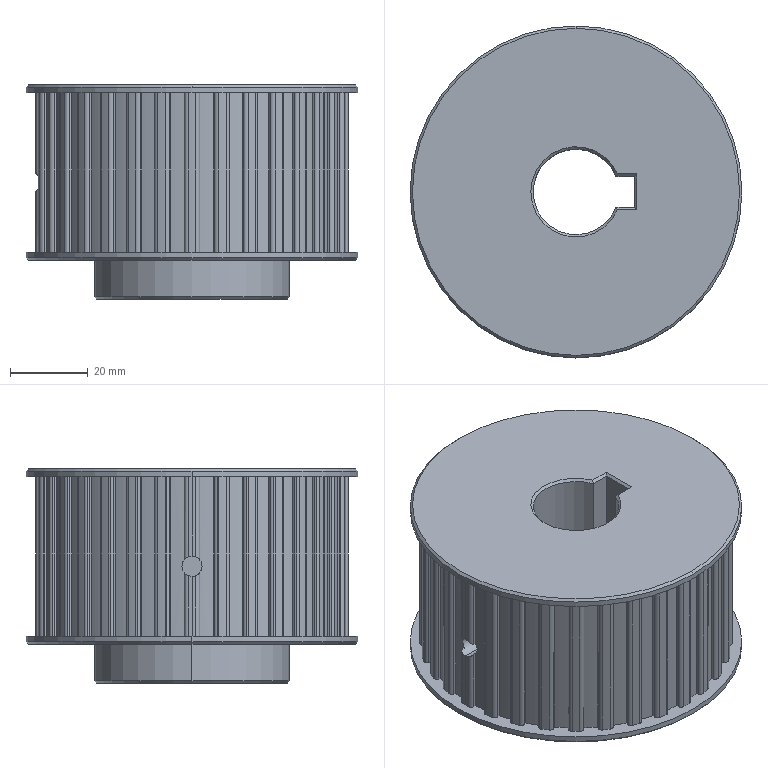Part | SolidWorks | features BaseBody 1 | 1 solid | 246 faces | box 85.12 x 85.12 x 55 mm | volume 217728 mm3 | cylinder 157 | plane 80 | cone 9 | commonest cylinder face diameters 2 x80 80.12 x35 77.12 x32 85.12 x4 5.2 x2 22 x2